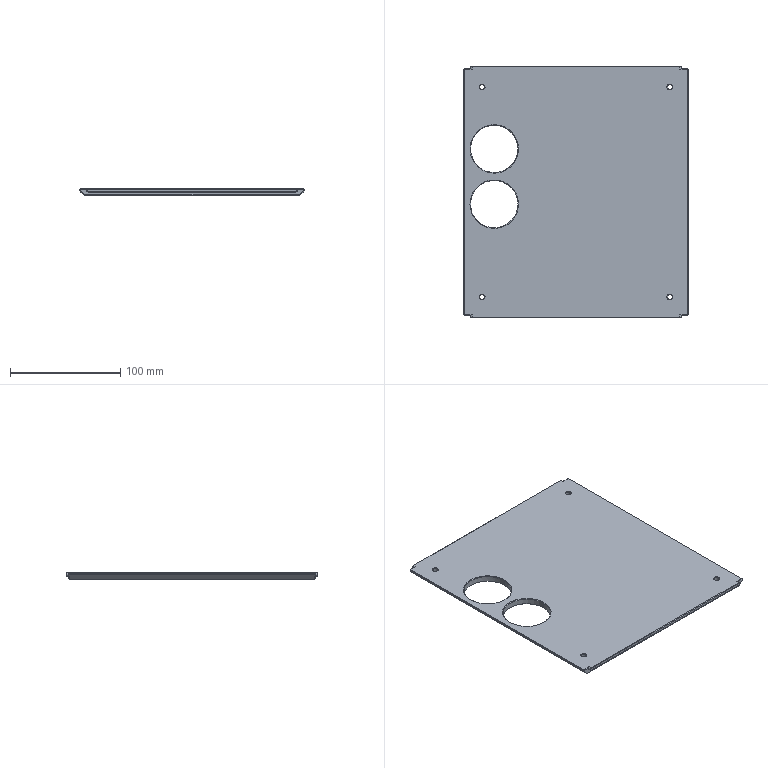Part | SolidWorks | features BaseBody 1 | 1 solid | 81 faces | box 203 x 228 x 6 mm | volume 252836 mm3 | plane 36 | cone 29 | cylinder 16 | commonest cylinder face diameters 4.3 x8 3 x4 43 x4